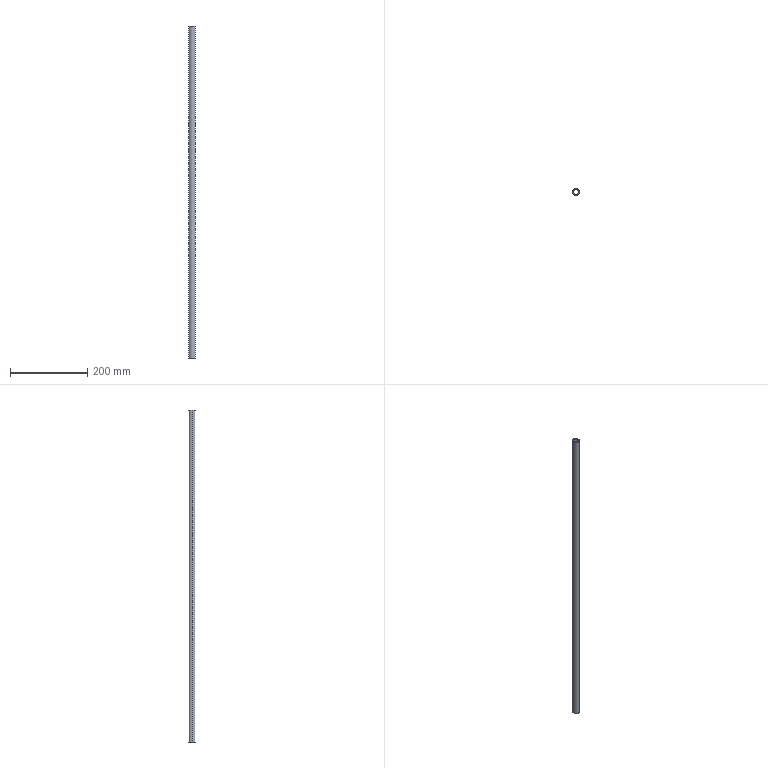Part | STEP file | 1 solid | 6 faces | box 18 x 18 x 860 mm | volume 104694 mm3 | cylinder 4 | plane 2 | commonest cylinder face diameters 13 x2 18 x2
STEP:
#1=CARTESIAN_POINT('',(0.,0.,0.));
#2=DIRECTION('',(0.,0.,1.));
#3=DIRECTION('',(1.,0.,0.));
#4=AXIS2_PLACEMENT_3D('',#1,#2,#3);
#5=CARTESIAN_POINT('',(-6.5,0.,0.));
#6=VERTEX_POINT('',#5);
#7=CARTESIAN_POINT('',(6.5,0.,0.));
#8=VERTEX_POINT('',#7);
#9=CARTESIAN_POINT('',(0.,0.,0.));
#10=DIRECTION('',(0.,0.,-1.));
#11=DIRECTION('',(-1.,0.,0.));
#12=AXIS2_PLACEMENT_3D('',#9,#10,#11);
#13=CIRCLE('',#12,6.5);
#14=CARTESIAN_POINT('',(0.,0.,860.));
#15=DIRECTION('',(0.,0.,-1.));
#16=DIRECTION('',(-1.,0.,0.));
#17=AXIS2_PLACEMENT_3D('',#14,#15,#16);
#18=CYLINDRICAL_SURFACE('',#17,6.5);
#19=CARTESIAN_POINT('',(0.,860.));
#20=DIRECTION('',(1.,0.));
#21=VECTOR('',#20,1.);
#22=LINE('',#19,#21);
#23=(GEOMETRIC_REPRESENTATION_CONTEXT(2)PARAMETRIC_REPRESENTATION_CONTEXT()REPRESENTATION_CONTEXT('',''));
#24=DEFINITIONAL_REPRESENTATION('',(#22),#23);
#25=PCURVE('',#18,#24);
#26=CARTESIAN_POINT('',(0.,0.,0.));
#27=DIRECTION('',(0.,0.,1.));
#28=DIRECTION('',(1.,0.,0.));
#29=AXIS2_PLACEMENT_3D('',#26,#27,#28);
#30=PLANE('',#29);
#31=CARTESIAN_POINT('',(-6.5,0.));
#32=CARTESIAN_POINT('',(-6.5,11.258));
#33=CARTESIAN_POINT('',(3.25,5.629));
#34=CARTESIAN_POINT('',(13.,0.));
#35=CARTESIAN_POINT('',(3.25,-5.629));
#36=CARTESIAN_POINT('',(-6.5,-11.258));
#37=CARTESIAN_POINT('',(-6.5,0.));
#38=(BOUNDED_CURVE()B_SPLINE_CURVE(2,(#31,#32,#33,#34,#35,#36,#37),.UNSPECIFIED.,.T.,.F.)B_SPLINE_CURVE_WITH_KNOTS((1,2,2,2,2,1),(-2.094,0.,2.094,4.189,6.283,8.378),.UNSPECIFIED.)CURVE()GEOMETRIC_REPRESENTATION_ITEM()RATIONAL_B_SPLINE_CURVE((1.,0.5,1.,0.5,1.,0.5,1.))REPRESENTATION_ITEM(''));
#39=(GEOMETRIC_REPRESENTATION_CONTEXT(2)PARAMETRIC_REPRESENTATION_CONTEXT()REPRESENTATION_CONTEXT('',''));
#40=DEFINITIONAL_REPRESENTATION('',(#38),#39);
#41=PCURVE('',#30,#40);
#42=SURFACE_CURVE('',#13,(#25,#41),.PCURVE_S1.);
#43=EDGE_CURVE('',#6,#8,#42,.T.);
#44=ORIENTED_EDGE('',*,*,#43,.F.);
#45=CARTESIAN_POINT('',(-6.5,0.,860.));
#46=VERTEX_POINT('',#45);
#47=CARTESIAN_POINT('',(-6.5,0.,860.));
#48=DIRECTION('',(0.,0.,-1.));
#49=VECTOR('',#48,1.);
#50=LINE('',#47,#49);
#51=CARTESIAN_POINT('',(0.,0.));
#52=DIRECTION('',(0.,1.));
#53=VECTOR('',#52,1.);
#54=LINE('',#51,#53);
#55=(GEOMETRIC_REPRESENTATION_CONTEXT(2)PARAMETRIC_REPRESENTATION_CONTEXT()REPRESENTATION_CONTEXT('',''));
#56=DEFINITIONAL_REPRESENTATION('',(#54),#55);
#57=PCURVE('',#18,#56);
#58=CARTESIAN_POINT('',(0.,0.,860.));
#59=DIRECTION('',(0.,0.,-1.));
#60=DIRECTION('',(-1.,0.,0.));
#61=AXIS2_PLACEMENT_3D('',#58,#59,#60);
#62=CYLINDRICAL_SURFACE('',#61,6.5);
#63=CARTESIAN_POINT('',(6.283,0.));
#64=DIRECTION('',(0.,1.));
#65=VECTOR('',#64,1.);
#66=LINE('',#63,#65);
#67=(GEOMETRIC_REPRESENTATION_CONTEXT(2)PARAMETRIC_REPRESENTATION_CONTEXT()REPRESENTATION_CONTEXT('',''));
#68=DEFINITIONAL_REPRESENTATION('',(#66),#67);
#69=PCURVE('',#62,#68);
#70=SURFACE_CURVE('',#50,(#57,#69),.PCURVE_S1.);
#71=EDGE_CURVE('',#46,#6,#70,.T.);
#72=ORIENTED_EDGE('',*,*,#71,.F.);
#73=CARTESIAN_POINT('',(6.5,0.,860.));
#74=VERTEX_POINT('',#73);
#75=CARTESIAN_POINT('',(0.,0.,860.));
#76=DIRECTION('',(0.,0.,-1.));
#77=DIRECTION('',(-1.,0.,0.));
#78=AXIS2_PLACEMENT_3D('',#75,#76,#77);
#79=CIRCLE('',#78,6.5);
#80=CARTESIAN_POINT('',(0.,0.));
#81=DIRECTION('',(1.,0.));
#82=VECTOR('',#81,1.);
#83=LINE('',#80,#82);
#84=(GEOMETRIC_REPRESENTATION_CONTEXT(2)PARAMETRIC_REPRESENTATION_CONTEXT()REPRESENTATION_CONTEXT('',''));
#85=DEFINITIONAL_REPRESENTATION('',(#83),#84);
#86=PCURVE('',#18,#85);
#87=CARTESIAN_POINT('',(0.,0.,860.));
#88=DIRECTION('',(0.,0.,1.));
#89=DIRECTION('',(1.,0.,0.));
#90=AXIS2_PLACEMENT_3D('',#87,#88,#89);
#91=PLANE('',#90);
#92=CARTESIAN_POINT('',(-6.5,0.));
#93=CARTESIAN_POINT('',(-6.5,11.258));
#94=CARTESIAN_POINT('',(3.25,5.629));
#95=CARTESIAN_POINT('',(13.,0.));
#96=CARTESIAN_POINT('',(3.25,-5.629));
#97=CARTESIAN_POINT('',(-6.5,-11.258));
#98=CARTESIAN_POINT('',(-6.5,0.));
#99=(BOUNDED_CURVE()B_SPLINE_CURVE(2,(#92,#93,#94,#95,#96,#97,#98),.UNSPECIFIED.,.T.,.F.)B_SPLINE_CURVE_WITH_KNOTS((1,2,2,2,2,1),(-2.094,0.,2.094,4.189,6.283,8.378),.UNSPECIFIED.)CURVE()GEOMETRIC_REPRESENTATION_ITEM()RATIONAL_B_SPLINE_CURVE((1.,0.5,1.,0.5,1.,0.5,1.))REPRESENTATION_ITEM(''));
#100=(GEOMETRIC_REPRESENTATION_CONTEXT(2)PARAMETRIC_REPRESENTATION_CONTEXT()REPRESENTATION_CONTEXT('',''));
#101=DEFINITIONAL_REPRESENTATION('',(#99),#100);
#102=PCURVE('',#91,#101);
#103=SURFACE_CURVE('',#79,(#86,#102),.PCURVE_S1.);
#104=EDGE_CURVE('',#46,#74,#103,.T.);
#105=ORIENTED_EDGE('',*,*,#104,.T.);
#106=CARTESIAN_POINT('',(6.5,0.,860.));
#107=DIRECTION('',(0.,0.,-1.));
#108=VECTOR('',#107,1.);
#109=LINE('',#106,#108);
#110=CARTESIAN_POINT('',(3.142,0.));
#111=DIRECTION('',(0.,1.));
#112=VECTOR('',#111,1.);
#113=LINE('',#110,#112);
#114=(GEOMETRIC_REPRESENTATION_CONTEXT(2)PARAMETRIC_REPRESENTATION_CONTEXT()REPRESENTATION_CONTEXT('',''));
#115=DEFINITIONAL_REPRESENTATION('',(#113),#114);
#116=PCURVE('',#18,#115);
#117=CARTESIAN_POINT('',(3.142,0.));
#118=DIRECTION('',(0.,1.));
#119=VECTOR('',#118,1.);
#120=LINE('',#117,#119);
#121=(GEOMETRIC_REPRESENTATION_CONTEXT(2)PARAMETRIC_REPRESENTATION_CONTEXT()REPRESENTATION_CONTEXT('',''));
#122=DEFINITIONAL_REPRESENTATION('',(#120),#121);
#123=PCURVE('',#62,#122);
#124=SURFACE_CURVE('',#109,(#116,#123),.PCURVE_S1.);
#125=EDGE_CURVE('',#74,#8,#124,.T.);
#126=ORIENTED_EDGE('',*,*,#125,.T.);
#127=EDGE_LOOP('',(#44,#72,#105,#126));
#128=FACE_BOUND('',#127,.F.);
#129=ADVANCED_FACE('',(#128),#18,.F.);
#130=ORIENTED_EDGE('',*,*,#104,.T.);
#131=CARTESIAN_POINT('',(0.,0.,860.));
#132=DIRECTION('',(0.,0.,-1.));
#133=DIRECTION('',(-1.,0.,0.));
#134=AXIS2_PLACEMENT_3D('',#131,#132,#133);
#135=CIRCLE('',#134,6.5);
#136=CARTESIAN_POINT('',(-6.5,0.));
#137=CARTESIAN_POINT('',(-6.5,11.258));
#138=CARTESIAN_POINT('',(3.25,5.629));
#139=CARTESIAN_POINT('',(13.,0.));
#140=CARTESIAN_POINT('',(3.25,-5.629));
#141=CARTESIAN_POINT('',(-6.5,-11.258));
#142=CARTESIAN_POINT('',(-6.5,0.));
#143=(BOUNDED_CURVE()B_SPLINE_CURVE(2,(#136,#137,#138,#139,#140,#141,#142),.UNSPECIFIED.,.T.,.F.)B_SPLINE_CURVE_WITH_KNOTS((1,2,2,2,2,1),(-2.094,0.,2.094,4.189,6.283,8.378),.UNSPECIFIED.)CURVE()GEOMETRIC_REPRESENTATION_ITEM()RATIONAL_B_SPLINE_CURVE((1.,0.5,1.,0.5,1.,0.5,1.))REPRESENTATION_ITEM(''));
#144=(GEOMETRIC_REPRESENTATION_CONTEXT(2)PARAMETRIC_REPRESENTATION_CONTEXT()REPRESENTATION_CONTEXT('',''));
#145=DEFINITIONAL_REPRESENTATION('',(#143),#144);
#146=PCURVE('',#91,#145);
#147=CARTESIAN_POINT('',(0.,0.));
#148=DIRECTION('',(1.,0.));
#149=VECTOR('',#148,1.);
#150=LINE('',#147,#149);
#151=(GEOMETRIC_REPRESENTATION_CONTEXT(2)PARAMETRIC_REPRESENTATION_CONTEXT()REPRESENTATION_CONTEXT('',''));
#152=DEFINITIONAL_REPRESENTATION('',(#150),#151);
#153=PCURVE('',#62,#152);
#154=SURFACE_CURVE('',#135,(#146,#153),.PCURVE_S1.);
#155=EDGE_CURVE('',#74,#46,#154,.T.);
#156=ORIENTED_EDGE('',*,*,#155,.T.);
#157=EDGE_LOOP('',(#130,#156));
#158=FACE_BOUND('',#157,.T.);
#159=CARTESIAN_POINT('',(-9.,0.,860.));
#160=VERTEX_POINT('',#159);
#161=CARTESIAN_POINT('',(9.,0.,860.));
#162=VERTEX_POINT('',#161);
#163=CARTESIAN_POINT('',(0.,0.,860.));
#164=DIRECTION('',(0.,0.,-1.));
#165=DIRECTION('',(-1.,0.,0.));
#166=AXIS2_PLACEMENT_3D('',#163,#164,#165);
#167=CIRCLE('',#166,9.);
#168=CARTESIAN_POINT('',(-9.,0.));
#169=CARTESIAN_POINT('',(-9.,15.588));
#170=CARTESIAN_POINT('',(4.5,7.794));
#171=CARTESIAN_POINT('',(18.,0.));
#172=CARTESIAN_POINT('',(4.5,-7.794));
#173=CARTESIAN_POINT('',(-9.,-15.588));
#174=CARTESIAN_POINT('',(-9.,0.));
#175=(BOUNDED_CURVE()B_SPLINE_CURVE(2,(#168,#169,#170,#171,#172,#173,#174),.UNSPECIFIED.,.T.,.F.)B_SPLINE_CURVE_WITH_KNOTS((1,2,2,2,2,1),(-2.094,0.,2.094,4.189,6.283,8.378),.UNSPECIFIED.)CURVE()GEOMETRIC_REPRESENTATION_ITEM()RATIONAL_B_SPLINE_CURVE((1.,0.5,1.,0.5,1.,0.5,1.))REPRESENTATION_ITEM(''));
#176=(GEOMETRIC_REPRESENTATION_CONTEXT(2)PARAMETRIC_REPRESENTATION_CONTEXT()REPRESENTATION_CONTEXT('',''));
#177=DEFINITIONAL_REPRESENTATION('',(#175),#176);
#178=PCURVE('',#91,#177);
#179=CARTESIAN_POINT('',(0.,0.,860.));
#180=DIRECTION('',(0.,0.,-1.));
#181=DIRECTION('',(-1.,0.,0.));
#182=AXIS2_PLACEMENT_3D('',#179,#180,#181);
#183=CYLINDRICAL_SURFACE('',#182,9.);
#184=CARTESIAN_POINT('',(0.,0.));
#185=DIRECTION('',(1.,0.));
#186=VECTOR('',#185,1.);
#187=LINE('',#184,#186);
#188=(GEOMETRIC_REPRESENTATION_CONTEXT(2)PARAMETRIC_REPRESENTATION_CONTEXT()REPRESENTATION_CONTEXT('',''));
#189=DEFINITIONAL_REPRESENTATION('',(#187),#188);
#190=PCURVE('',#183,#189);
#191=SURFACE_CURVE('',#167,(#178,#190),.PCURVE_S1.);
#192=EDGE_CURVE('',#160,#162,#191,.T.);
#193=ORIENTED_EDGE('',*,*,#192,.F.);
#194=CARTESIAN_POINT('',(0.,0.,860.));
#195=DIRECTION('',(0.,0.,-1.));
#196=DIRECTION('',(-1.,0.,0.));
#197=AXIS2_PLACEMENT_3D('',#194,#195,#196);
#198=CIRCLE('',#197,9.);
#199=CARTESIAN_POINT('',(-9.,0.));
#200=CARTESIAN_POINT('',(-9.,15.588));
#201=CARTESIAN_POINT('',(4.5,7.794));
#202=CARTESIAN_POINT('',(18.,0.));
#203=CARTESIAN_POINT('',(4.5,-7.794));
#204=CARTESIAN_POINT('',(-9.,-15.588));
#205=CARTESIAN_POINT('',(-9.,0.));
#206=(BOUNDED_CURVE()B_SPLINE_CURVE(2,(#199,#200,#201,#202,#203,#204,#205),.UNSPECIFIED.,.T.,.F.)B_SPLINE_CURVE_WITH_KNOTS((1,2,2,2,2,1),(-2.094,0.,2.094,4.189,6.283,8.378),.UNSPECIFIED.)CURVE()GEOMETRIC_REPRESENTATION_ITEM()RATIONAL_B_SPLINE_CURVE((1.,0.5,1.,0.5,1.,0.5,1.))REPRESENTATION_ITEM(''));
#207=(GEOMETRIC_REPRESENTATION_CONTEXT(2)PARAMETRIC_REPRESENTATION_CONTEXT()REPRESENTATION_CONTEXT('',''));
#208=DEFINITIONAL_REPRESENTATION('',(#206),#207);
#209=PCURVE('',#91,#208);
#210=CARTESIAN_POINT('',(0.,0.,860.));
#211=DIRECTION('',(0.,0.,-1.));
#212=DIRECTION('',(-1.,0.,0.));
#213=AXIS2_PLACEMENT_3D('',#210,#211,#212);
#214=CYLINDRICAL_SURFACE('',#213,9.);
#215=CARTESIAN_POINT('',(0.,0.));
#216=DIRECTION('',(1.,0.));
#217=VECTOR('',#216,1.);
#218=LINE('',#215,#217);
#219=(GEOMETRIC_REPRESENTATION_CONTEXT(2)PARAMETRIC_REPRESENTATION_CONTEXT()REPRESENTATION_CONTEXT('',''));
#220=DEFINITIONAL_REPRESENTATION('',(#218),#219);
#221=PCURVE('',#214,#220);
#222=SURFACE_CURVE('',#198,(#209,#221),.PCURVE_S1.);
#223=EDGE_CURVE('',#162,#160,#222,.T.);
#224=ORIENTED_EDGE('',*,*,#223,.F.);
#225=EDGE_LOOP('',(#193,#224));
#226=FACE_BOUND('',#225,.T.);
#227=ADVANCED_FACE('',(#158,#226),#91,.T.);
#228=ORIENTED_EDGE('',*,*,#43,.F.);
#229=CARTESIAN_POINT('',(0.,0.,0.));
#230=DIRECTION('',(0.,0.,-1.));
#231=DIRECTION('',(-1.,0.,0.));
#232=AXIS2_PLACEMENT_3D('',#229,#230,#231);
#233=CIRCLE('',#232,6.5);
#234=CARTESIAN_POINT('',(-6.5,0.));
#235=CARTESIAN_POINT('',(-6.5,11.258));
#236=CARTESIAN_POINT('',(3.25,5.629));
#237=CARTESIAN_POINT('',(13.,0.));
#238=CARTESIAN_POINT('',(3.25,-5.629));
#239=CARTESIAN_POINT('',(-6.5,-11.258));
#240=CARTESIAN_POINT('',(-6.5,0.));
#241=(BOUNDED_CURVE()B_SPLINE_CURVE(2,(#234,#235,#236,#237,#238,#239,#240),.UNSPECIFIED.,.T.,.F.)B_SPLINE_CURVE_WITH_KNOTS((1,2,2,2,2,1),(-2.094,0.,2.094,4.189,6.283,8.378),.UNSPECIFIED.)CURVE()GEOMETRIC_REPRESENTATION_ITEM()RATIONAL_B_SPLINE_CURVE((1.,0.5,1.,0.5,1.,0.5,1.))REPRESENTATION_ITEM(''));
#242=(GEOMETRIC_REPRESENTATION_CONTEXT(2)PARAMETRIC_REPRESENTATION_CONTEXT()REPRESENTATION_CONTEXT('',''));
#243=DEFINITIONAL_REPRESENTATION('',(#241),#242);
#244=PCURVE('',#30,#243);
#245=CARTESIAN_POINT('',(0.,860.));
#246=DIRECTION('',(1.,0.));
#247=VECTOR('',#246,1.);
#248=LINE('',#245,#247);
#249=(GEOMETRIC_REPRESENTATION_CONTEXT(2)PARAMETRIC_REPRESENTATION_CONTEXT()REPRESENTATION_CONTEXT('',''));
#250=DEFINITIONAL_REPRESENTATION('',(#248),#249);
#251=PCURVE('',#62,#250);
#252=SURFACE_CURVE('',#233,(#244,#251),.PCURVE_S1.);
#253=EDGE_CURVE('',#8,#6,#252,.T.);
#254=ORIENTED_EDGE('',*,*,#253,.F.);
#255=EDGE_LOOP('',(#228,#254));
#256=FACE_BOUND('',#255,.T.);
#257=CARTESIAN_POINT('',(-9.,0.,0.));
#258=VERTEX_POINT('',#257);
#259=CARTESIAN_POINT('',(9.,0.,0.));
#260=VERTEX_POINT('',#259);
#261=CARTESIAN_POINT('',(0.,0.,0.));
#262=DIRECTION('',(0.,0.,1.));
#263=DIRECTION('',(-1.,0.,0.));
#264=AXIS2_PLACEMENT_3D('',#261,#262,#263);
#265=CIRCLE('',#264,9.);
#266=CARTESIAN_POINT('',(0.,0.));
#267=DIRECTION('',(-1.,0.));
#268=AXIS2_PLACEMENT_2D('',#266,#267);
#269=CIRCLE('',#268,9.);
#270=(GEOMETRIC_REPRESENTATION_CONTEXT(2)PARAMETRIC_REPRESENTATION_CONTEXT()REPRESENTATION_CONTEXT('',''));
#271=DEFINITIONAL_REPRESENTATION('',(#269),#270);
#272=PCURVE('',#30,#271);
#273=CARTESIAN_POINT('',(6.283,860.));
#274=DIRECTION('',(-1.,0.));
#275=VECTOR('',#274,1.);
#276=LINE('',#273,#275);
#277=(GEOMETRIC_REPRESENTATION_CONTEXT(2)PARAMETRIC_REPRESENTATION_CONTEXT()REPRESENTATION_CONTEXT('',''));
#278=DEFINITIONAL_REPRESENTATION('',(#276),#277);
#279=PCURVE('',#214,#278);
#280=SURFACE_CURVE('',#265,(#272,#279),.PCURVE_S1.);
#281=EDGE_CURVE('',#258,#260,#280,.T.);
#282=ORIENTED_EDGE('',*,*,#281,.F.);
#283=CARTESIAN_POINT('',(0.,0.,0.));
#284=DIRECTION('',(0.,0.,1.));
#285=DIRECTION('',(-1.,0.,0.));
#286=AXIS2_PLACEMENT_3D('',#283,#284,#285);
#287=CIRCLE('',#286,9.);
#288=CARTESIAN_POINT('',(0.,0.));
#289=DIRECTION('',(-1.,0.));
#290=AXIS2_PLACEMENT_2D('',#288,#289);
#291=CIRCLE('',#290,9.);
#292=(GEOMETRIC_REPRESENTATION_CONTEXT(2)PARAMETRIC_REPRESENTATION_CONTEXT()REPRESENTATION_CONTEXT('',''));
#293=DEFINITIONAL_REPRESENTATION('',(#291),#292);
#294=PCURVE('',#30,#293);
#295=CARTESIAN_POINT('',(6.283,860.));
#296=DIRECTION('',(-1.,0.));
#297=VECTOR('',#296,1.);
#298=LINE('',#295,#297);
#299=(GEOMETRIC_REPRESENTATION_CONTEXT(2)PARAMETRIC_REPRESENTATION_CONTEXT()REPRESENTATION_CONTEXT('',''));
#300=DEFINITIONAL_REPRESENTATION('',(#298),#299);
#301=PCURVE('',#183,#300);
#302=SURFACE_CURVE('',#287,(#294,#301),.PCURVE_S1.);
#303=EDGE_CURVE('',#260,#258,#302,.T.);
#304=ORIENTED_EDGE('',*,*,#303,.F.);
#305=EDGE_LOOP('',(#282,#304));
#306=FACE_BOUND('',#305,.T.);
#307=ADVANCED_FACE('',(#256,#306),#30,.F.);
#308=CARTESIAN_POINT('',(9.,0.,860.));
#309=DIRECTION('',(0.,0.,-1.));
#310=VECTOR('',#309,1.);
#311=LINE('',#308,#310);
#312=CARTESIAN_POINT('',(3.142,0.));
#313=DIRECTION('',(0.,1.));
#314=VECTOR('',#313,1.);
#315=LINE('',#312,#314);
#316=(GEOMETRIC_REPRESENTATION_CONTEXT(2)PARAMETRIC_REPRESENTATION_CONTEXT()REPRESENTATION_CONTEXT('',''));
#317=DEFINITIONAL_REPRESENTATION('',(#315),#316);
#318=PCURVE('',#214,#317);
#319=CARTESIAN_POINT('',(3.142,0.));
#320=DIRECTION('',(0.,1.));
#321=VECTOR('',#320,1.);
#322=LINE('',#319,#321);
#323=(GEOMETRIC_REPRESENTATION_CONTEXT(2)PARAMETRIC_REPRESENTATION_CONTEXT()REPRESENTATION_CONTEXT('',''));
#324=DEFINITIONAL_REPRESENTATION('',(#322),#323);
#325=PCURVE('',#183,#324);
#326=SURFACE_CURVE('',#311,(#318,#325),.PCURVE_S1.);
#327=EDGE_CURVE('',#162,#260,#326,.T.);
#328=ORIENTED_EDGE('',*,*,#327,.F.);
#329=ORIENTED_EDGE('',*,*,#223,.T.);
#330=CARTESIAN_POINT('',(-9.,0.,860.));
#331=DIRECTION('',(0.,0.,-1.));
#332=VECTOR('',#331,1.);
#333=LINE('',#330,#332);
#334=CARTESIAN_POINT('',(6.283,0.));
#335=DIRECTION('',(0.,1.));
#336=VECTOR('',#335,1.);
#337=LINE('',#334,#336);
#338=(GEOMETRIC_REPRESENTATION_CONTEXT(2)PARAMETRIC_REPRESENTATION_CONTEXT()REPRESENTATION_CONTEXT('',''));
#339=DEFINITIONAL_REPRESENTATION('',(#337),#338);
#340=PCURVE('',#214,#339);
#341=CARTESIAN_POINT('',(0.,0.));
#342=DIRECTION('',(0.,1.));
#343=VECTOR('',#342,1.);
#344=LINE('',#341,#343);
#345=(GEOMETRIC_REPRESENTATION_CONTEXT(2)PARAMETRIC_REPRESENTATION_CONTEXT()REPRESENTATION_CONTEXT('',''));
#346=DEFINITIONAL_REPRESENTATION('',(#344),#345);
#347=PCURVE('',#183,#346);
#348=SURFACE_CURVE('',#333,(#340,#347),.PCURVE_S1.);
#349=EDGE_CURVE('',#160,#258,#348,.T.);
#350=ORIENTED_EDGE('',*,*,#349,.T.);
#351=ORIENTED_EDGE('',*,*,#281,.T.);
#352=EDGE_LOOP('',(#328,#329,#350,#351));
#353=FACE_BOUND('',#352,.T.);
#354=ADVANCED_FACE('',(#353),#214,.T.);
#355=ORIENTED_EDGE('',*,*,#71,.T.);
#356=ORIENTED_EDGE('',*,*,#253,.F.);
#357=ORIENTED_EDGE('',*,*,#125,.F.);
#358=ORIENTED_EDGE('',*,*,#155,.T.);
#359=EDGE_LOOP('',(#355,#356,#357,#358));
#360=FACE_BOUND('',#359,.F.);
#361=ADVANCED_FACE('',(#360),#62,.F.);
#362=ORIENTED_EDGE('',*,*,#192,.T.);
#363=ORIENTED_EDGE('',*,*,#327,.T.);
#364=ORIENTED_EDGE('',*,*,#303,.T.);
#365=ORIENTED_EDGE('',*,*,#349,.F.);
#366=EDGE_LOOP('',(#362,#363,#364,#365));
#367=FACE_BOUND('',#366,.T.);
#368=ADVANCED_FACE('',(#367),#183,.T.);
#369=CLOSED_SHELL('',(#129,#227,#307,#354,#361,#368));
#370=MANIFOLD_SOLID_BREP('',#369);
#371=(LENGTH_UNIT()NAMED_UNIT(*)SI_UNIT(.MILLI.,.METRE.));
#372=UNCERTAINTY_MEASURE_WITH_UNIT(LENGTH_MEASURE(0.0000001),#371,'','');
#373=(NAMED_UNIT(*)PLANE_ANGLE_UNIT()SI_UNIT($,.RADIAN.));
#374=(NAMED_UNIT(*)SI_UNIT($,.STERADIAN.)SOLID_ANGLE_UNIT());
#375=(GEOMETRIC_REPRESENTATION_CONTEXT(3)GLOBAL_UNCERTAINTY_ASSIGNED_CONTEXT((#372))GLOBAL_UNIT_ASSIGNED_CONTEXT((#371,#373,#374))REPRESENTATION_CONTEXT('',''));
#376=ADVANCED_BREP_SHAPE_REPRESENTATION('',(#4,#370),#375);